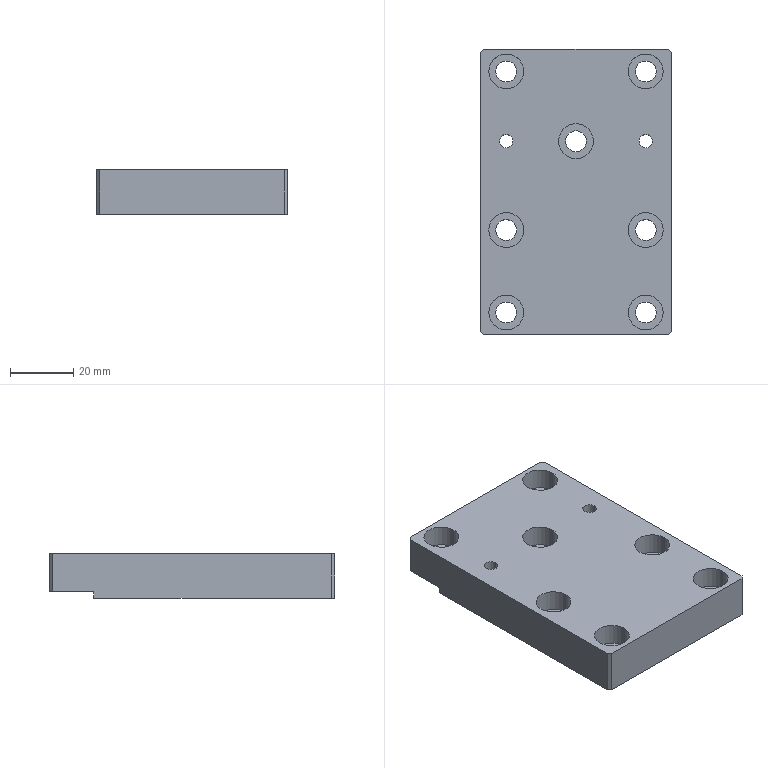Part | SolidWorks | features HoleWzd 2, Chamfer 1, Extrusion 1, ICE 1 | 1 solid | 51 faces | box 60 x 90 x 14 mm | volume 67395 mm3 | cylinder 32 | plane 19 | commonest cylinder face diameters 6.6 x14 11 x14 4.2 x4
STEP:
#1=CARTESIAN_POINT('',(-24.1,16.,-7.));
#2=VERTEX_POINT('',#1);
#3=CARTESIAN_POINT('',(-19.9,16.,-7.));
#4=VERTEX_POINT('',#3);
#5=CARTESIAN_POINT('',(-22.,16.,-7.));
#6=DIRECTION('',(0.,0.,1.));
#7=DIRECTION('',(1.,0.,0.));
#8=AXIS2_PLACEMENT_3D('',#5,#6,#7);
#9=CIRCLE('',#8,2.1);
#10=EDGE_CURVE('',#2,#4,#9,.T.);
#11=ORIENTED_EDGE('',*,*,#10,.F.);
#12=CARTESIAN_POINT('',(-24.1,16.,7.));
#13=VERTEX_POINT('',#12);
#14=CARTESIAN_POINT('',(-24.1,16.,7.));
#15=DIRECTION('',(0.,0.,1.));
#16=VECTOR('',#15,1000.);
#17=LINE('',#14,#16);
#18=EDGE_CURVE('',#2,#13,#17,.T.);
#19=ORIENTED_EDGE('',*,*,#18,.T.);
#20=CARTESIAN_POINT('',(-19.9,16.,7.));
#21=VERTEX_POINT('',#20);
#22=CARTESIAN_POINT('',(-22.,16.,7.));
#23=DIRECTION('',(0.,0.,1.));
#24=DIRECTION('',(1.,0.,0.));
#25=AXIS2_PLACEMENT_3D('',#22,#23,#24);
#26=CIRCLE('',#25,2.1);
#27=EDGE_CURVE('',#13,#21,#26,.T.);
#28=ORIENTED_EDGE('',*,*,#27,.T.);
#29=CARTESIAN_POINT('',(-19.9,16.,7.));
#30=DIRECTION('',(0.,0.,1.));
#31=VECTOR('',#30,1000.);
#32=LINE('',#29,#31);
#33=EDGE_CURVE('',#4,#21,#32,.T.);
#34=ORIENTED_EDGE('',*,*,#33,.F.);
#35=EDGE_LOOP('',(#11,#19,#28,#34));
#36=FACE_OUTER_BOUND('',#35,.T.);
#37=CARTESIAN_POINT('',(-22.,16.,7.));
#38=DIRECTION('',(0.,0.,1.));
#39=DIRECTION('',(1.,0.,0.));
#40=AXIS2_PLACEMENT_3D('',#37,#38,#39);
#41=CYLINDRICAL_SURFACE('',#40,2.1);
#42=ADVANCED_FACE('',(#36),#41,.F.);
#43=CARTESIAN_POINT('',(19.9,16.,-7.));
#44=VERTEX_POINT('',#43);
#45=CARTESIAN_POINT('',(24.1,16.,-7.));
#46=VERTEX_POINT('',#45);
#47=CARTESIAN_POINT('',(22.,16.,-7.));
#48=DIRECTION('',(0.,0.,1.));
#49=DIRECTION('',(1.,0.,0.));
#50=AXIS2_PLACEMENT_3D('',#47,#48,#49);
#51=CIRCLE('',#50,2.1);
#52=EDGE_CURVE('',#44,#46,#51,.T.);
#53=ORIENTED_EDGE('',*,*,#52,.F.);
#54=CARTESIAN_POINT('',(19.9,16.,7.));
#55=VERTEX_POINT('',#54);
#56=CARTESIAN_POINT('',(19.9,16.,7.));
#57=DIRECTION('',(0.,0.,1.));
#58=VECTOR('',#57,1000.);
#59=LINE('',#56,#58);
#60=EDGE_CURVE('',#44,#55,#59,.T.);
#61=ORIENTED_EDGE('',*,*,#60,.T.);
#62=CARTESIAN_POINT('',(24.1,16.,7.));
#63=VERTEX_POINT('',#62);
#64=CARTESIAN_POINT('',(22.,16.,7.));
#65=DIRECTION('',(0.,0.,1.));
#66=DIRECTION('',(1.,0.,0.));
#67=AXIS2_PLACEMENT_3D('',#64,#65,#66);
#68=CIRCLE('',#67,2.1);
#69=EDGE_CURVE('',#55,#63,#68,.T.);
#70=ORIENTED_EDGE('',*,*,#69,.T.);
#71=CARTESIAN_POINT('',(24.1,16.,7.));
#72=DIRECTION('',(0.,0.,1.));
#73=VECTOR('',#72,1000.);
#74=LINE('',#71,#73);
#75=EDGE_CURVE('',#46,#63,#74,.T.);
#76=ORIENTED_EDGE('',*,*,#75,.F.);
#77=EDGE_LOOP('',(#53,#61,#70,#76));
#78=FACE_OUTER_BOUND('',#77,.T.);
#79=CARTESIAN_POINT('',(22.,16.,7.));
#80=DIRECTION('',(0.,0.,1.));
#81=DIRECTION('',(1.,0.,0.));
#82=AXIS2_PLACEMENT_3D('',#79,#80,#81);
#83=CYLINDRICAL_SURFACE('',#82,2.1);
#84=ADVANCED_FACE('',(#78),#83,.F.);
#85=CARTESIAN_POINT('',(-27.5,38.,0.2));
#86=VERTEX_POINT('',#85);
#87=CARTESIAN_POINT('',(-16.5,38.,0.2));
#88=VERTEX_POINT('',#87);
#89=CARTESIAN_POINT('',(-22.,38.,0.2));
#90=DIRECTION('',(0.,0.,1.));
#91=DIRECTION('',(1.,0.,0.));
#92=AXIS2_PLACEMENT_3D('',#89,#90,#91);
#93=CIRCLE('',#92,5.5);
#94=EDGE_CURVE('',#86,#88,#93,.T.);
#95=ORIENTED_EDGE('',*,*,#94,.F.);
#96=CARTESIAN_POINT('',(-27.5,38.,7.));
#97=VERTEX_POINT('',#96);
#98=CARTESIAN_POINT('',(-27.5,38.,7.));
#99=DIRECTION('',(0.,0.,1.));
#100=VECTOR('',#99,1000.);
#101=LINE('',#98,#100);
#102=EDGE_CURVE('',#86,#97,#101,.T.);
#103=ORIENTED_EDGE('',*,*,#102,.T.);
#104=CARTESIAN_POINT('',(-16.5,38.,7.));
#105=VERTEX_POINT('',#104);
#106=CARTESIAN_POINT('',(-22.,38.,7.));
#107=DIRECTION('',(0.,0.,1.));
#108=DIRECTION('',(1.,0.,0.));
#109=AXIS2_PLACEMENT_3D('',#106,#107,#108);
#110=CIRCLE('',#109,5.5);
#111=EDGE_CURVE('',#97,#105,#110,.T.);
#112=ORIENTED_EDGE('',*,*,#111,.T.);
#113=CARTESIAN_POINT('',(-16.5,38.,7.));
#114=DIRECTION('',(0.,0.,1.));
#115=VECTOR('',#114,1000.);
#116=LINE('',#113,#115);
#117=EDGE_CURVE('',#88,#105,#116,.T.);
#118=ORIENTED_EDGE('',*,*,#117,.F.);
#119=EDGE_LOOP('',(#95,#103,#112,#118));
#120=FACE_OUTER_BOUND('',#119,.T.);
#121=CARTESIAN_POINT('',(-22.,38.,7.));
#122=DIRECTION('',(0.,0.,1.));
#123=DIRECTION('',(1.,0.,0.));
#124=AXIS2_PLACEMENT_3D('',#121,#122,#123);
#125=CYLINDRICAL_SURFACE('',#124,5.5);
#126=ADVANCED_FACE('',(#120),#125,.F.);
#127=CARTESIAN_POINT('',(-18.7,38.,-5.));
#128=VERTEX_POINT('',#127);
#129=CARTESIAN_POINT('',(-25.3,38.,-5.));
#130=VERTEX_POINT('',#129);
#131=CARTESIAN_POINT('',(-22.,38.,-5.));
#132=DIRECTION('',(0.,0.,-1.));
#133=DIRECTION('',(-1.,0.,0.));
#134=AXIS2_PLACEMENT_3D('',#131,#132,#133);
#135=CIRCLE('',#134,3.3);
#136=EDGE_CURVE('',#128,#130,#135,.T.);
#137=ORIENTED_EDGE('',*,*,#136,.T.);
#138=CARTESIAN_POINT('',(-25.3,38.,0.2));
#139=VERTEX_POINT('',#138);
#140=CARTESIAN_POINT('',(-25.3,38.,7.));
#141=DIRECTION('',(0.,0.,1.));
#142=VECTOR('',#141,1000.);
#143=LINE('',#140,#142);
#144=EDGE_CURVE('',#130,#139,#143,.T.);
#145=ORIENTED_EDGE('',*,*,#144,.T.);
#146=CARTESIAN_POINT('',(-18.7,38.,0.2));
#147=VERTEX_POINT('',#146);
#148=CARTESIAN_POINT('',(-22.,38.,0.2));
#149=DIRECTION('',(0.,0.,1.));
#150=DIRECTION('',(1.,0.,0.));
#151=AXIS2_PLACEMENT_3D('',#148,#149,#150);
#152=CIRCLE('',#151,3.3);
#153=EDGE_CURVE('',#139,#147,#152,.T.);
#154=ORIENTED_EDGE('',*,*,#153,.T.);
#155=CARTESIAN_POINT('',(-18.7,38.,7.));
#156=DIRECTION('',(0.,0.,1.));
#157=VECTOR('',#156,1000.);
#158=LINE('',#155,#157);
#159=EDGE_CURVE('',#128,#147,#158,.T.);
#160=ORIENTED_EDGE('',*,*,#159,.F.);
#161=EDGE_LOOP('',(#137,#145,#154,#160));
#162=FACE_OUTER_BOUND('',#161,.T.);
#163=CARTESIAN_POINT('',(-22.,38.,7.));
#164=DIRECTION('',(0.,0.,1.));
#165=DIRECTION('',(1.,0.,0.));
#166=AXIS2_PLACEMENT_3D('',#163,#164,#165);
#167=CYLINDRICAL_SURFACE('',#166,3.3);
#168=ADVANCED_FACE('',(#162),#167,.F.);
#169=CARTESIAN_POINT('',(16.5,38.,0.2));
#170=VERTEX_POINT('',#169);
#171=CARTESIAN_POINT('',(27.5,38.,0.2));
#172=VERTEX_POINT('',#171);
#173=CARTESIAN_POINT('',(22.,38.,0.2));
#174=DIRECTION('',(0.,0.,1.));
#175=DIRECTION('',(1.,0.,0.));
#176=AXIS2_PLACEMENT_3D('',#173,#174,#175);
#177=CIRCLE('',#176,5.5);
#178=EDGE_CURVE('',#170,#172,#177,.T.);
#179=ORIENTED_EDGE('',*,*,#178,.F.);
#180=CARTESIAN_POINT('',(16.5,38.,7.));
#181=VERTEX_POINT('',#180);
#182=CARTESIAN_POINT('',(16.5,38.,7.));
#183=DIRECTION('',(0.,0.,1.));
#184=VECTOR('',#183,1000.);
#185=LINE('',#182,#184);
#186=EDGE_CURVE('',#170,#181,#185,.T.);
#187=ORIENTED_EDGE('',*,*,#186,.T.);
#188=CARTESIAN_POINT('',(27.5,38.,7.));
#189=VERTEX_POINT('',#188);
#190=CARTESIAN_POINT('',(22.,38.,7.));
#191=DIRECTION('',(0.,0.,1.));
#192=DIRECTION('',(1.,0.,0.));
#193=AXIS2_PLACEMENT_3D('',#190,#191,#192);
#194=CIRCLE('',#193,5.5);
#195=EDGE_CURVE('',#181,#189,#194,.T.);
#196=ORIENTED_EDGE('',*,*,#195,.T.);
#197=CARTESIAN_POINT('',(27.5,38.,7.));
#198=DIRECTION('',(0.,0.,1.));
#199=VECTOR('',#198,1000.);
#200=LINE('',#197,#199);
#201=EDGE_CURVE('',#172,#189,#200,.T.);
#202=ORIENTED_EDGE('',*,*,#201,.F.);
#203=EDGE_LOOP('',(#179,#187,#196,#202));
#204=FACE_OUTER_BOUND('',#203,.T.);
#205=CARTESIAN_POINT('',(22.,38.,7.));
#206=DIRECTION('',(0.,0.,1.));
#207=DIRECTION('',(1.,0.,0.));
#208=AXIS2_PLACEMENT_3D('',#205,#206,#207);
#209=CYLINDRICAL_SURFACE('',#208,5.5);
#210=ADVANCED_FACE('',(#204),#209,.F.);
#211=CARTESIAN_POINT('',(25.3,38.,-5.));
#212=VERTEX_POINT('',#211);
#213=CARTESIAN_POINT('',(18.7,38.,-5.));
#214=VERTEX_POINT('',#213);
#215=CARTESIAN_POINT('',(22.,38.,-5.));
#216=DIRECTION('',(0.,0.,-1.));
#217=DIRECTION('',(-1.,0.,0.));
#218=AXIS2_PLACEMENT_3D('',#215,#216,#217);
#219=CIRCLE('',#218,3.3);
#220=EDGE_CURVE('',#212,#214,#219,.T.);
#221=ORIENTED_EDGE('',*,*,#220,.T.);
#222=CARTESIAN_POINT('',(18.7,38.,0.2));
#223=VERTEX_POINT('',#222);
#224=CARTESIAN_POINT('',(18.7,38.,7.));
#225=DIRECTION('',(0.,0.,1.));
#226=VECTOR('',#225,1000.);
#227=LINE('',#224,#226);
#228=EDGE_CURVE('',#214,#223,#227,.T.);
#229=ORIENTED_EDGE('',*,*,#228,.T.);
#230=CARTESIAN_POINT('',(25.3,38.,0.2));
#231=VERTEX_POINT('',#230);
#232=CARTESIAN_POINT('',(22.,38.,0.2));
#233=DIRECTION('',(0.,0.,1.));
#234=DIRECTION('',(1.,0.,0.));
#235=AXIS2_PLACEMENT_3D('',#232,#233,#234);
#236=CIRCLE('',#235,3.3);
#237=EDGE_CURVE('',#223,#231,#236,.T.);
#238=ORIENTED_EDGE('',*,*,#237,.T.);
#239=CARTESIAN_POINT('',(25.3,38.,7.));
#240=DIRECTION('',(0.,0.,1.));
#241=VECTOR('',#240,1000.);
#242=LINE('',#239,#241);
#243=EDGE_CURVE('',#212,#231,#242,.T.);
#244=ORIENTED_EDGE('',*,*,#243,.F.);
#245=EDGE_LOOP('',(#221,#229,#238,#244));
#246=FACE_OUTER_BOUND('',#245,.T.);
#247=CARTESIAN_POINT('',(22.,38.,7.));
#248=DIRECTION('',(0.,0.,1.));
#249=DIRECTION('',(1.,0.,0.));
#250=AXIS2_PLACEMENT_3D('',#247,#248,#249);
#251=CYLINDRICAL_SURFACE('',#250,3.3);
#252=ADVANCED_FACE('',(#246),#251,.F.);
#253=CARTESIAN_POINT('',(-27.5,-12.,0.2));
#254=VERTEX_POINT('',#253);
#255=CARTESIAN_POINT('',(-16.5,-12.,0.2));
#256=VERTEX_POINT('',#255);
#257=CARTESIAN_POINT('',(-22.,-12.,0.2));
#258=DIRECTION('',(0.,0.,1.));
#259=DIRECTION('',(1.,0.,0.));
#260=AXIS2_PLACEMENT_3D('',#257,#258,#259);
#261=CIRCLE('',#260,5.5);
#262=EDGE_CURVE('',#254,#256,#261,.T.);
#263=ORIENTED_EDGE('',*,*,#262,.F.);
#264=CARTESIAN_POINT('',(-27.5,-12.,7.));
#265=VERTEX_POINT('',#264);
#266=CARTESIAN_POINT('',(-27.5,-12.,7.));
#267=DIRECTION('',(0.,0.,1.));
#268=VECTOR('',#267,1000.);
#269=LINE('',#266,#268);
#270=EDGE_CURVE('',#254,#265,#269,.T.);
#271=ORIENTED_EDGE('',*,*,#270,.T.);
#272=CARTESIAN_POINT('',(-16.5,-12.,7.));
#273=VERTEX_POINT('',#272);
#274=CARTESIAN_POINT('',(-22.,-12.,7.));
#275=DIRECTION('',(0.,0.,1.));
#276=DIRECTION('',(1.,0.,0.));
#277=AXIS2_PLACEMENT_3D('',#274,#275,#276);
#278=CIRCLE('',#277,5.5);
#279=EDGE_CURVE('',#265,#273,#278,.T.);
#280=ORIENTED_EDGE('',*,*,#279,.T.);
#281=CARTESIAN_POINT('',(-16.5,-12.,7.));
#282=DIRECTION('',(0.,0.,1.));
#283=VECTOR('',#282,1000.);
#284=LINE('',#281,#283);
#285=EDGE_CURVE('',#256,#273,#284,.T.);
#286=ORIENTED_EDGE('',*,*,#285,.F.);
#287=EDGE_LOOP('',(#263,#271,#280,#286));
#288=FACE_OUTER_BOUND('',#287,.T.);
#289=CARTESIAN_POINT('',(-22.,-12.,7.));
#290=DIRECTION('',(0.,0.,1.));
#291=DIRECTION('',(1.,0.,0.));
#292=AXIS2_PLACEMENT_3D('',#289,#290,#291);
#293=CYLINDRICAL_SURFACE('',#292,5.5);
#294=ADVANCED_FACE('',(#288),#293,.F.);
#295=CARTESIAN_POINT('',(-25.3,-12.,-7.));
#296=VERTEX_POINT('',#295);
#297=CARTESIAN_POINT('',(-18.7,-12.,-7.));
#298=VERTEX_POINT('',#297);
#299=CARTESIAN_POINT('',(-22.,-12.,-7.));
#300=DIRECTION('',(0.,0.,1.));
#301=DIRECTION('',(1.,0.,0.));
#302=AXIS2_PLACEMENT_3D('',#299,#300,#301);
#303=CIRCLE('',#302,3.3);
#304=EDGE_CURVE('',#296,#298,#303,.T.);
#305=ORIENTED_EDGE('',*,*,#304,.F.);
#306=CARTESIAN_POINT('',(-25.3,-12.,0.2));
#307=VERTEX_POINT('',#306);
#308=CARTESIAN_POINT('',(-25.3,-12.,7.));
#309=DIRECTION('',(0.,0.,1.));
#310=VECTOR('',#309,1000.);
#311=LINE('',#308,#310);
#312=EDGE_CURVE('',#296,#307,#311,.T.);
#313=ORIENTED_EDGE('',*,*,#312,.T.);
#314=CARTESIAN_POINT('',(-18.7,-12.,0.2));
#315=VERTEX_POINT('',#314);
#316=CARTESIAN_POINT('',(-22.,-12.,0.2));
#317=DIRECTION('',(0.,0.,1.));
#318=DIRECTION('',(1.,0.,0.));
#319=AXIS2_PLACEMENT_3D('',#316,#317,#318);
#320=CIRCLE('',#319,3.3);
#321=EDGE_CURVE('',#307,#315,#320,.T.);
#322=ORIENTED_EDGE('',*,*,#321,.T.);
#323=CARTESIAN_POINT('',(-18.7,-12.,7.));
#324=DIRECTION('',(0.,0.,1.));
#325=VECTOR('',#324,1000.);
#326=LINE('',#323,#325);
#327=EDGE_CURVE('',#298,#315,#326,.T.);
#328=ORIENTED_EDGE('',*,*,#327,.F.);
#329=EDGE_LOOP('',(#305,#313,#322,#328));
#330=FACE_OUTER_BOUND('',#329,.T.);
#331=CARTESIAN_POINT('',(-22.,-12.,7.));
#332=DIRECTION('',(0.,0.,1.));
#333=DIRECTION('',(1.,0.,0.));
#334=AXIS2_PLACEMENT_3D('',#331,#332,#333);
#335=CYLINDRICAL_SURFACE('',#334,3.3);
#336=ADVANCED_FACE('',(#330),#335,.F.);
#337=CARTESIAN_POINT('',(16.5,-38.,0.2));
#338=VERTEX_POINT('',#337);
#339=CARTESIAN_POINT('',(27.5,-38.,0.2));
#340=VERTEX_POINT('',#339);
#341=CARTESIAN_POINT('',(22.,-38.,0.2));
#342=DIRECTION('',(0.,0.,1.));
#343=DIRECTION('',(1.,0.,0.));
#344=AXIS2_PLACEMENT_3D('',#341,#342,#343);
#345=CIRCLE('',#344,5.5);
#346=EDGE_CURVE('',#338,#340,#345,.T.);
#347=ORIENTED_EDGE('',*,*,#346,.F.);
#348=CARTESIAN_POINT('',(16.5,-38.,7.));
#349=VERTEX_POINT('',#348);
#350=CARTESIAN_POINT('',(16.5,-38.,7.));
#351=DIRECTION('',(0.,0.,1.));
#352=VECTOR('',#351,1000.);
#353=LINE('',#350,#352);
#354=EDGE_CURVE('',#338,#349,#353,.T.);
#355=ORIENTED_EDGE('',*,*,#354,.T.);
#356=CARTESIAN_POINT('',(27.5,-38.,7.));
#357=VERTEX_POINT('',#356);
#358=CARTESIAN_POINT('',(22.,-38.,7.));
#359=DIRECTION('',(0.,0.,1.));
#360=DIRECTION('',(1.,0.,0.));
#361=AXIS2_PLACEMENT_3D('',#358,#359,#360);
#362=CIRCLE('',#361,5.5);
#363=EDGE_CURVE('',#349,#357,#362,.T.);
#364=ORIENTED_EDGE('',*,*,#363,.T.);
#365=CARTESIAN_POINT('',(27.5,-38.,7.));
#366=DIRECTION('',(0.,0.,1.));
#367=VECTOR('',#366,1000.);
#368=LINE('',#365,#367);
#369=EDGE_CURVE('',#340,#357,#368,.T.);
#370=ORIENTED_EDGE('',*,*,#369,.F.);
#371=EDGE_LOOP('',(#347,#355,#364,#370));
#372=FACE_OUTER_BOUND('',#371,.T.);
#373=CARTESIAN_POINT('',(22.,-38.,7.));
#374=DIRECTION('',(0.,0.,1.));
#375=DIRECTION('',(1.,0.,0.));
#376=AXIS2_PLACEMENT_3D('',#373,#374,#375);
#377=CYLINDRICAL_SURFACE('',#376,5.5);
#378=ADVANCED_FACE('',(#372),#377,.F.);
#379=CARTESIAN_POINT('',(18.7,-38.,-7.));
#380=VERTEX_POINT('',#379);
#381=CARTESIAN_POINT('',(25.3,-38.,-7.));
#382=VERTEX_POINT('',#381);
#383=CARTESIAN_POINT('',(22.,-38.,-7.));
#384=DIRECTION('',(0.,0.,1.));
#385=DIRECTION('',(1.,0.,0.));
#386=AXIS2_PLACEMENT_3D('',#383,#384,#385);
#387=CIRCLE('',#386,3.3);
#388=EDGE_CURVE('',#380,#382,#387,.T.);
#389=ORIENTED_EDGE('',*,*,#388,.F.);
#390=CARTESIAN_POINT('',(18.7,-38.,0.2));
#391=VERTEX_POINT('',#390);
#392=CARTESIAN_POINT('',(18.7,-38.,7.));
#393=DIRECTION('',(0.,0.,1.));
#394=VECTOR('',#393,1000.);
#395=LINE('',#392,#394);
#396=EDGE_CURVE('',#380,#391,#395,.T.);
#397=ORIENTED_EDGE('',*,*,#396,.T.);
#398=CARTESIAN_POINT('',(25.3,-38.,0.2));
#399=VERTEX_POINT('',#398);
#400=CARTESIAN_POINT('',(22.,-38.,0.2));
#401=DIRECTION('',(0.,0.,1.));
#402=DIRECTION('',(1.,0.,0.));
#403=AXIS2_PLACEMENT_3D('',#400,#401,#402);
#404=CIRCLE('',#403,3.3);
#405=EDGE_CURVE('',#391,#399,#404,.T.);
#406=ORIENTED_EDGE('',*,*,#405,.T.);
#407=CARTESIAN_POINT('',(25.3,-38.,7.));
#408=DIRECTION('',(0.,0.,1.));
#409=VECTOR('',#408,1000.);
#410=LINE('',#407,#409);
#411=EDGE_CURVE('',#382,#399,#410,.T.);
#412=ORIENTED_EDGE('',*,*,#411,.F.);
#413=EDGE_LOOP('',(#389,#397,#406,#412));
#414=FACE_OUTER_BOUND('',#413,.T.);
#415=CARTESIAN_POINT('',(22.,-38.,7.));
#416=DIRECTION('',(0.,0.,1.));
#417=DIRECTION('',(1.,0.,0.));
#418=AXIS2_PLACEMENT_3D('',#415,#416,#417);
#419=CYLINDRICAL_SURFACE('',#418,3.3);
#420=ADVANCED_FACE('',(#414),#419,.F.);
#421=CARTESIAN_POINT('',(-27.5,-38.,0.2));
#422=VERTEX_POINT('',#421);
#423=CARTESIAN_POINT('',(-16.5,-38.,0.2));
#424=VERTEX_POINT('',#423);
#425=CARTESIAN_POINT('',(-22.,-38.,0.2));
#426=DIRECTION('',(0.,0.,1.));
#427=DIRECTION('',(1.,0.,0.));
#428=AXIS2_PLACEMENT_3D('',#425,#426,#427);
#429=CIRCLE('',#428,5.5);
#430=EDGE_CURVE('',#422,#424,#429,.T.);
#431=ORIENTED_EDGE('',*,*,#430,.F.);
#432=CARTESIAN_POINT('',(-27.5,-38.,7.));
#433=VERTEX_POINT('',#432);
#434=CARTESIAN_POINT('',(-27.5,-38.,7.));
#435=DIRECTION('',(0.,0.,1.));
#436=VECTOR('',#435,1000.);
#437=LINE('',#434,#436);
#438=EDGE_CURVE('',#422,#433,#437,.T.);
#439=ORIENTED_EDGE('',*,*,#438,.T.);
#440=CARTESIAN_POINT('',(-16.5,-38.,7.));
#441=VERTEX_POINT('',#440);
#442=CARTESIAN_POINT('',(-22.,-38.,7.));
#443=DIRECTION('',(0.,0.,1.));
#444=DIRECTION('',(1.,0.,0.));
#445=AXIS2_PLACEMENT_3D('',#442,#443,#444);
#446=CIRCLE('',#445,5.5);
#447=EDGE_CURVE('',#433,#441,#446,.T.);
#448=ORIENTED_EDGE('',*,*,#447,.T.);
#449=CARTESIAN_POINT('',(-16.5,-38.,7.));
#450=DIRECTION('',(0.,0.,1.));
#451=VECTOR('',#450,1000.);
#452=LINE('',#449,#451);
#453=EDGE_CURVE('',#424,#441,#452,.T.);
#454=ORIENTED_EDGE('',*,*,#453,.F.);
#455=EDGE_LOOP('',(#431,#439,#448,#454));
#456=FACE_OUTER_BOUND('',#455,.T.);
#457=CARTESIAN_POINT('',(-22.,-38.,7.));
#458=DIRECTION('',(0.,0.,1.));
#459=DIRECTION('',(1.,0.,0.));
#460=AXIS2_PLACEMENT_3D('',#457,#458,#459);
#461=CYLINDRICAL_SURFACE('',#460,5.5);
#462=ADVANCED_FACE('',(#456),#461,.F.);
#463=CARTESIAN_POINT('',(-25.3,-38.,-7.));
#464=VERTEX_POINT('',#463);
#465=CARTESIAN_POINT('',(-18.7,-38.,-7.));
#466=VERTEX_POINT('',#465);
#467=CARTESIAN_POINT('',(-22.,-38.,-7.));
#468=DIRECTION('',(0.,0.,1.));
#469=DIRECTION('',(1.,0.,0.));
#470=AXIS2_PLACEMENT_3D('',#467,#468,#469);
#471=CIRCLE('',#470,3.3);
#472=EDGE_CURVE('',#464,#466,#471,.T.);
#473=ORIENTED_EDGE('',*,*,#472,.F.);
#474=CARTESIAN_POINT('',(-25.3,-38.,0.2));
#475=VERTEX_POINT('',#474);
#476=CARTESIAN_POINT('',(-25.3,-38.,7.));
#477=DIRECTION('',(0.,0.,1.));
#478=VECTOR('',#477,1000.);
#479=LINE('',#476,#478);
#480=EDGE_CURVE('',#464,#475,#479,.T.);
#481=ORIENTED_EDGE('',*,*,#480,.T.);
#482=CARTESIAN_POINT('',(-18.7,-38.,0.2));
#483=VERTEX_POINT('',#482);
#484=CARTESIAN_POINT('',(-22.,-38.,0.2));
#485=DIRECTION('',(0.,0.,1.));
#486=DIRECTION('',(1.,0.,0.));
#487=AXIS2_PLACEMENT_3D('',#484,#485,#486);
#488=CIRCLE('',#487,3.3);
#489=EDGE_CURVE('',#475,#483,#488,.T.);
#490=ORIENTED_EDGE('',*,*,#489,.T.);
#491=CARTESIAN_POINT('',(-18.7,-38.,7.));
#492=DIRECTION('',(0.,0.,1.));
#493=VECTOR('',#492,1000.);
#494=LINE('',#491,#493);
#495=EDGE_CURVE('',#466,#483,#494,.T.);
#496=ORIENTED_EDGE('',*,*,#495,.F.);
#497=EDGE_LOOP('',(#473,#481,#490,#496));
#498=FACE_OUTER_BOUND('',#497,.T.);
#499=CARTESIAN_POINT('',(-22.,-38.,7.));
#500=DIRECTION('',(0.,0.,1.));
#501=DIRECTION('',(1.,0.,0.));
#502=AXIS2_PLACEMENT_3D('',#499,#500,#501);
#503=CYLINDRICAL_SURFACE('',#502,3.3);
#504=ADVANCED_FACE('',(#498),#503,.F.);
#505=CARTESIAN_POINT('',(16.5,-12.,0.2));
#506=VERTEX_POINT('',#505);
#507=CARTESIAN_POINT('',(27.5,-12.,0.2));
#508=VERTEX_POINT('',#507);
#509=CARTESIAN_POINT('',(22.,-12.,0.2));
#510=DIRECTION('',(0.,0.,1.));
#511=DIRECTION('',(1.,0.,0.));
#512=AXIS2_PLACEMENT_3D('',#509,#510,#511);
#513=CIRCLE('',#512,5.5);
#514=EDGE_CURVE('',#506,#508,#513,.T.);
#515=ORIENTED_EDGE('',*,*,#514,.F.);
#516=CARTESIAN_POINT('',(16.5,-12.,7.));
#517=VERTEX_POINT('',#516);
#518=CARTESIAN_POINT('',(16.5,-12.,7.));
#519=DIRECTION('',(0.,0.,1.));
#520=VECTOR('',#519,1000.);
#521=LINE('',#518,#520);
#522=EDGE_CURVE('',#506,#517,#521,.T.);
#523=ORIENTED_EDGE('',*,*,#522,.T.);
#524=CARTESIAN_POINT('',(27.5,-12.,7.));
#525=VERTEX_POINT('',#524);
#526=CARTESIAN_POINT('',(22.,-12.,7.));
#527=DIRECTION('',(0.,0.,1.));
#528=DIRECTION('',(1.,0.,0.));
#529=AXIS2_PLACEMENT_3D('',#526,#527,#528);
#530=CIRCLE('',#529,5.5);
#531=EDGE_CURVE('',#517,#525,#530,.T.);
#532=ORIENTED_EDGE('',*,*,#531,.T.);
#533=CARTESIAN_POINT('',(27.5,-12.,7.));
#534=DIRECTION('',(0.,0.,1.));
#535=VECTOR('',#534,1000.);
#536=LINE('',#533,#535);
#537=EDGE_CURVE('',#508,#525,#536,.T.);
#538=ORIENTED_EDGE('',*,*,#537,.F.);
#539=EDGE_LOOP('',(#515,#523,#532,#538));
#540=FACE_OUTER_BOUND('',#539,.T.);
#541=CARTESIAN_POINT('',(22.,-12.,7.));
#542=DIRECTION('',(0.,0.,1.));
#543=DIRECTION('',(1.,0.,0.));
#544=AXIS2_PLACEMENT_3D('',#541,#542,#543);
#545=CYLINDRICAL_SURFACE('',#544,5.5);
#546=ADVANCED_FACE('',(#540),#545,.F.);
#547=CARTESIAN_POINT('',(18.7,-12.,-7.));
#548=VERTEX_POINT('',#547);
#549=CARTESIAN_POINT('',(25.3,-12.,-7.));
#550=VERTEX_POINT('',#549);
#551=CARTESIAN_POINT('',(22.,-12.,-7.));
#552=DIRECTION('',(0.,0.,1.));
#553=DIRECTION('',(1.,0.,0.));
#554=AXIS2_PLACEMENT_3D('',#551,#552,#553);
#555=CIRCLE('',#554,3.3);
#556=EDGE_CURVE('',#548,#550,#555,.T.);
#557=ORIENTED_EDGE('',*,*,#556,.F.);
#558=CARTESIAN_POINT('',(18.7,-12.,0.2));
#559=VERTEX_POINT('',#558);
#560=CARTESIAN_POINT('',(18.7,-12.,7.));
#561=DIRECTION('',(0.,0.,1.));
#562=VECTOR('',#561,1000.);
#563=LINE('',#560,#562);
#564=EDGE_CURVE('',#548,#559,#563,.T.);
#565=ORIENTED_EDGE('',*,*,#564,.T.);
#566=CARTESIAN_POINT('',(25.3,-12.,0.2));
#567=VERTEX_POINT('',#566);
#568=CARTESIAN_POINT('',(22.,-12.,0.2));
#569=DIRECTION('',(0.,0.,1.));
#570=DIRECTION('',(1.,0.,0.));
#571=AXIS2_PLACEMENT_3D('',#568,#569,#570);
#572=CIRCLE('',#571,3.3);
#573=EDGE_CURVE('',#559,#567,#572,.T.);
#574=ORIENTED_EDGE('',*,*,#573,.T.);
#575=CARTESIAN_POINT('',(25.3,-12.,7.));
#576=DIRECTION('',(0.,0.,1.));
#577=VECTOR('',#576,1000.);
#578=LINE('',#575,#577);
#579=EDGE_CURVE('',#550,#567,#578,.T.);
#580=ORIENTED_EDGE('',*,*,#579,.F.);
#581=EDGE_LOOP('',(#557,#565,#574,#580));
#582=FACE_OUTER_BOUND('',#581,.T.);
#583=CARTESIAN_POINT('',(22.,-12.,7.));
#584=DIRECTION('',(0.,0.,1.));
#585=DIRECTION('',(1.,0.,0.));
#586=AXIS2_PLACEMENT_3D('',#583,#584,#585);
#587=CYLINDRICAL_SURFACE('',#586,3.3);
#588=ADVANCED_FACE('',(#582),#587,.F.);
#589=CARTESIAN_POINT('',(-5.5,16.,0.2));
#590=VERTEX_POINT('',#589);
#591=CARTESIAN_POINT('',(5.5,16.,0.2));
#592=VERTEX_POINT('',#591);
#593=CARTESIAN_POINT('',(0.,16.,0.2));
#594=DIRECTION('',(0.,0.,1.));
#595=DIRECTION('',(1.,0.,0.));
#596=AXIS2_PLACEMENT_3D('',#593,#594,#595);
#597=CIRCLE('',#596,5.5);
#598=EDGE_CURVE('',#590,#592,#597,.T.);
#599=ORIENTED_EDGE('',*,*,#598,.F.);
#600=CARTESIAN_POINT('',(-5.5,16.,7.));
#601=VERTEX_POINT('',#600);
#602=CARTESIAN_POINT('',(-5.5,16.,7.));
#603=DIRECTION('',(0.,0.,1.));
#604=VECTOR('',#603,1000.);
#605=LINE('',#602,#604);
#606=EDGE_CURVE('',#590,#601,#605,.T.);
#607=ORIENTED_EDGE('',*,*,#606,.T.);
#608=CARTESIAN_POINT('',(5.5,16.,7.));
#609=VERTEX_POINT('',#608);
#610=CARTESIAN_POINT('',(0.,16.,7.));
#611=DIRECTION('',(0.,0.,1.));
#612=DIRECTION('',(1.,0.,0.));
#613=AXIS2_PLACEMENT_3D('',#610,#611,#612);
#614=CIRCLE('',#613,5.5);
#615=EDGE_CURVE('',#601,#609,#614,.T.);
#616=ORIENTED_EDGE('',*,*,#615,.T.);
#617=CARTESIAN_POINT('',(5.5,16.,7.));
#618=DIRECTION('',(0.,0.,1.));
#619=VECTOR('',#618,1000.);
#620=LINE('',#617,#619);
#621=EDGE_CURVE('',#592,#609,#620,.T.);
#622=ORIENTED_EDGE('',*,*,#621,.F.);
#623=EDGE_LOOP('',(#599,#607,#616,#622));
#624=FACE_OUTER_BOUND('',#623,.T.);
#625=CARTESIAN_POINT('',(0.,16.,7.));
#626=DIRECTION('',(0.,0.,1.));
#627=DIRECTION('',(1.,0.,0.));
#628=AXIS2_PLACEMENT_3D('',#625,#626,#627);
#629=CYLINDRICAL_SURFACE('',#628,5.5);
#630=ADVANCED_FACE('',(#624),#629,.F.);
#631=CARTESIAN_POINT('',(-3.3,16.,-7.));
#632=VERTEX_POINT('',#631);
#633=CARTESIAN_POINT('',(3.3,16.,-7.));
#634=VERTEX_POINT('',#633);
#635=CARTESIAN_POINT('',(0.,16.,-7.));
#636=DIRECTION('',(0.,0.,1.));
#637=DIRECTION('',(1.,0.,0.));
#638=AXIS2_PLACEMENT_3D('',#635,#636,#637);
#639=CIRCLE('',#638,3.3);
#640=EDGE_CURVE('',#632,#634,#639,.T.);
#641=ORIENTED_EDGE('',*,*,#640,.F.);
#642=CARTESIAN_POINT('',(-3.3,16.,0.2));
#643=VERTEX_POINT('',#642);
#644=CARTESIAN_POINT('',(-3.3,16.,7.));
#645=DIRECTION('',(0.,0.,1.));
#646=VECTOR('',#645,1000.);
#647=LINE('',#644,#646);
#648=EDGE_CURVE('',#632,#643,#647,.T.);
#649=ORIENTED_EDGE('',*,*,#648,.T.);
#650=CARTESIAN_POINT('',(3.3,16.,0.2));
#651=VERTEX_POINT('',#650);
#652=CARTESIAN_POINT('',(0.,16.,0.2));
#653=DIRECTION('',(0.,0.,1.));
#654=DIRECTION('',(1.,0.,0.));
#655=AXIS2_PLACEMENT_3D('',#652,#653,#654);
#656=CIRCLE('',#655,3.3);
#657=EDGE_CURVE('',#643,#651,#656,.T.);
#658=ORIENTED_EDGE('',*,*,#657,.T.);
#659=CARTESIAN_POINT('',(3.3,16.,7.));
#660=DIRECTION('',(0.,0.,1.));
#661=VECTOR('',#660,1000.);
#662=LINE('',#659,#661);
#663=EDGE_CURVE('',#634,#651,#662,.T.);
#664=ORIENTED_EDGE('',*,*,#663,.F.);
#665=EDGE_LOOP('',(#641,#649,#658,#664));
#666=FACE_OUTER_BOUND('',#665,.T.);
#667=CARTESIAN_POINT('',(0.,16.,7.));
#668=DIRECTION('',(0.,0.,1.));
#669=DIRECTION('',(1.,0.,0.));
#670=AXIS2_PLACEMENT_3D('',#667,#668,#669);
#671=CYLINDRICAL_SURFACE('',#670,3.3);
#672=ADVANCED_FACE('',(#666),#671,.F.);
#673=CARTESIAN_POINT('',(29.,45.,7.));
#674=VERTEX_POINT('',#673);
#675=CARTESIAN_POINT('',(-29.,45.,7.));
#676=VERTEX_POINT('',#675);
#677=CARTESIAN_POINT('',(-30.,45.,7.));
#678=DIRECTION('',(-1.,0.,0.));
#679=VECTOR('',#678,1000.);
#680=LINE('',#677,#679);
#681=EDGE_CURVE('',#674,#676,#680,.T.);
#682=ORIENTED_EDGE('',*,*,#681,.F.);
#683=CARTESIAN_POINT('',(29.,45.,-5.));
#684=VERTEX_POINT('',#683);
#685=CARTESIAN_POINT('',(29.,45.,7.));
#686=DIRECTION('',(0.,0.,-1.));
#687=VECTOR('',#686,1000.);
#688=LINE('',#685,#687);
#689=EDGE_CURVE('',#674,#684,#688,.T.);
#690=ORIENTED_EDGE('',*,*,#689,.T.);
#691=CARTESIAN_POINT('',(-29.,45.,-5.));
#692=VERTEX_POINT('',#691);
#693=CARTESIAN_POINT('',(30.,45.,-5.));
#694=DIRECTION('',(1.,0.,0.));
#695=VECTOR('',#694,1000.);
#696=LINE('',#693,#695);
#697=EDGE_CURVE('',#692,#684,#696,.T.);
#698=ORIENTED_EDGE('',*,*,#697,.F.);
#699=CARTESIAN_POINT('',(-29.,45.,7.));
#700=DIRECTION('',(0.,0.,1.));
#701=VECTOR('',#700,1000.);
#702=LINE('',#699,#701);
#703=EDGE_CURVE('',#692,#676,#702,.T.);
#704=ORIENTED_EDGE('',*,*,#703,.T.);
#705=EDGE_LOOP('',(#682,#690,#698,#704));
#706=FACE_OUTER_BOUND('',#705,.T.);
#707=CARTESIAN_POINT('',(-30.,45.,7.));
#708=DIRECTION('',(0.,-1.,0.));
#709=DIRECTION('',(0.,0.,-1.));
#710=AXIS2_PLACEMENT_3D('',#707,#708,#709);
#711=PLANE('',#710);
#712=ADVANCED_FACE('',(#706),#711,.F.);
#713=CARTESIAN_POINT('',(30.,-44.,7.));
#714=VERTEX_POINT('',#713);
#715=CARTESIAN_POINT('',(30.,44.,7.));
#716=VERTEX_POINT('',#715);
#717=CARTESIAN_POINT('',(30.,-45.,7.));
#718=DIRECTION('',(0.,1.,0.));
#719=VECTOR('',#718,1000.);
#720=LINE('',#717,#719);
#721=EDGE_CURVE('',#714,#716,#720,.T.);
#722=ORIENTED_EDGE('',*,*,#721,.F.);
#723=CARTESIAN_POINT('',(30.,-44.,-7.));
#724=VERTEX_POINT('',#723);
#725=CARTESIAN_POINT('',(30.,-44.,7.));
#726=DIRECTION('',(0.,0.,-1.));
#727=VECTOR('',#726,1000.);
#728=LINE('',#725,#727);
#729=EDGE_CURVE('',#714,#724,#728,.T.);
#730=ORIENTED_EDGE('',*,*,#729,.T.);
#731=CARTESIAN_POINT('',(30.,31.,-7.));
#732=VERTEX_POINT('',#731);
#733=CARTESIAN_POINT('',(30.,-45.,-7.));
#734=DIRECTION('',(0.,1.,0.));
#735=VECTOR('',#734,1000.);
#736=LINE('',#733,#735);
#737=EDGE_CURVE('',#724,#732,#736,.T.);
#738=ORIENTED_EDGE('',*,*,#737,.T.);
#739=CARTESIAN_POINT('',(30.,31.,-5.));
#740=VERTEX_POINT('',#739);
#741=CARTESIAN_POINT('',(30.,31.,-5.));
#742=DIRECTION('',(0.,0.,-1.));
#743=VECTOR('',#742,1000.);
#744=LINE('',#741,#743);
#745=EDGE_CURVE('',#740,#732,#744,.T.);
#746=ORIENTED_EDGE('',*,*,#745,.F.);
#747=CARTESIAN_POINT('',(30.,44.,-5.));
#748=VERTEX_POINT('',#747);
#749=CARTESIAN_POINT('',(30.,45.,-5.));
#750=DIRECTION('',(0.,-1.,0.));
#751=VECTOR('',#750,1000.);
#752=LINE('',#749,#751);
#753=EDGE_CURVE('',#748,#740,#752,.T.);
#754=ORIENTED_EDGE('',*,*,#753,.F.);
#755=CARTESIAN_POINT('',(30.,44.,7.));
#756=DIRECTION('',(0.,0.,1.));
#757=VECTOR('',#756,1000.);
#758=LINE('',#755,#757);
#759=EDGE_CURVE('',#748,#716,#758,.T.);
#760=ORIENTED_EDGE('',*,*,#759,.T.);
#761=EDGE_LOOP('',(#722,#730,#738,#746,#754,#760));
#762=FACE_OUTER_BOUND('',#761,.T.);
#763=CARTESIAN_POINT('',(30.,-45.,7.));
#764=DIRECTION('',(-1.,0.,0.));
#765=DIRECTION('',(0.,0.,1.));
#766=AXIS2_PLACEMENT_3D('',#763,#764,#765);
#767=PLANE('',#766);
#768=ADVANCED_FACE('',(#762),#767,.F.);
#769=CARTESIAN_POINT('',(-30.,31.,-7.));
#770=VERTEX_POINT('',#769);
#771=CARTESIAN_POINT('',(-30.,-44.,-7.));
#772=VERTEX_POINT('',#771);
#773=CARTESIAN_POINT('',(-30.,-45.,-7.));
#774=DIRECTION('',(0.,-1.,0.));
#775=VECTOR('',#774,1000.);
#776=LINE('',#773,#775);
#777=EDGE_CURVE('',#770,#772,#776,.T.);
#778=ORIENTED_EDGE('',*,*,#777,.T.);
#779=CARTESIAN_POINT('',(-30.,-44.,7.));
#780=VERTEX_POINT('',#779);
#781=CARTESIAN_POINT('',(-30.,-44.,7.));
#782=DIRECTION('',(0.,0.,1.));
#783=VECTOR('',#782,1000.);
#784=LINE('',#781,#783);
#785=EDGE_CURVE('',#772,#780,#784,.T.);
#786=ORIENTED_EDGE('',*,*,#785,.T.);
#787=CARTESIAN_POINT('',(-30.,44.,7.));
#788=VERTEX_POINT('',#787);
#789=CARTESIAN_POINT('',(-30.,-45.,7.));
#790=DIRECTION('',(0.,-1.,0.));
#791=VECTOR('',#790,1000.);
#792=LINE('',#789,#791);
#793=EDGE_CURVE('',#788,#780,#792,.T.);
#794=ORIENTED_EDGE('',*,*,#793,.F.);
#795=CARTESIAN_POINT('',(-30.,44.,-5.));
#796=VERTEX_POINT('',#795);
#797=CARTESIAN_POINT('',(-30.,44.,7.));
#798=DIRECTION('',(0.,0.,-1.));
#799=VECTOR('',#798,1000.);
#800=LINE('',#797,#799);
#801=EDGE_CURVE('',#788,#796,#800,.T.);
#802=ORIENTED_EDGE('',*,*,#801,.T.);
#803=CARTESIAN_POINT('',(-30.,31.,-5.));
#804=VERTEX_POINT('',#803);
#805=CARTESIAN_POINT('',(-30.,45.,-5.));
#806=DIRECTION('',(0.,1.,0.));
#807=VECTOR('',#806,1000.);
#808=LINE('',#805,#807);
#809=EDGE_CURVE('',#804,#796,#808,.T.);
#810=ORIENTED_EDGE('',*,*,#809,.F.);
#811=CARTESIAN_POINT('',(-30.,31.,-5.));
#812=DIRECTION('',(0.,0.,-1.));
#813=VECTOR('',#812,1000.);
#814=LINE('',#811,#813);
#815=EDGE_CURVE('',#804,#770,#814,.T.);
#816=ORIENTED_EDGE('',*,*,#815,.T.);
#817=EDGE_LOOP('',(#778,#786,#794,#802,#810,#816));
#818=FACE_OUTER_BOUND('',#817,.T.);
#819=CARTESIAN_POINT('',(-30.,-45.,7.));
#820=DIRECTION('',(1.,0.,0.));
#821=DIRECTION('',(0.,0.,-1.));
#822=AXIS2_PLACEMENT_3D('',#819,#820,#821);
#823=PLANE('',#822);
#824=ADVANCED_FACE('',(#818),#823,.F.);
#825=CARTESIAN_POINT('',(-29.,-45.,-7.));
#826=VERTEX_POINT('',#825);
#827=CARTESIAN_POINT('',(29.,-45.,-7.));
#828=VERTEX_POINT('',#827);
#829=CARTESIAN_POINT('',(-30.,-45.,-7.));
#830=DIRECTION('',(1.,0.,0.));
#831=VECTOR('',#830,1000.);
#832=LINE('',#829,#831);
#833=EDGE_CURVE('',#826,#828,#832,.T.);
#834=ORIENTED_EDGE('',*,*,#833,.T.);
#835=CARTESIAN_POINT('',(29.,-45.,7.));
#836=VERTEX_POINT('',#835);
#837=CARTESIAN_POINT('',(29.,-45.,7.));
#838=DIRECTION('',(0.,0.,1.));
#839=VECTOR('',#838,1000.);
#840=LINE('',#837,#839);
#841=EDGE_CURVE('',#828,#836,#840,.T.);
#842=ORIENTED_EDGE('',*,*,#841,.T.);
#843=CARTESIAN_POINT('',(-29.,-45.,7.));
#844=VERTEX_POINT('',#843);
#845=CARTESIAN_POINT('',(-30.,-45.,7.));
#846=DIRECTION('',(1.,0.,0.));
#847=VECTOR('',#846,1000.);
#848=LINE('',#845,#847);
#849=EDGE_CURVE('',#844,#836,#848,.T.);
#850=ORIENTED_EDGE('',*,*,#849,.F.);
#851=CARTESIAN_POINT('',(-29.,-45.,7.));
#852=DIRECTION('',(0.,0.,-1.));
#853=VECTOR('',#852,1000.);
#854=LINE('',#851,#853);
#855=EDGE_CURVE('',#844,#826,#854,.T.);
#856=ORIENTED_EDGE('',*,*,#855,.T.);
#857=EDGE_LOOP('',(#834,#842,#850,#856));
#858=FACE_OUTER_BOUND('',#857,.T.);
#859=CARTESIAN_POINT('',(-30.,-45.,7.));
#860=DIRECTION('',(0.,1.,0.));
#861=DIRECTION('',(0.,0.,1.));
#862=AXIS2_PLACEMENT_3D('',#859,#860,#861);
#863=PLANE('',#862);
#864=ADVANCED_FACE('',(#858),#863,.F.);
#865=CARTESIAN_POINT('',(-22.,16.,7.));
#866=DIRECTION('',(0.,0.,1.));
#867=DIRECTION('',(1.,0.,0.));
#868=AXIS2_PLACEMENT_3D('',#865,#866,#867);
#869=CIRCLE('',#868,2.1);
#870=EDGE_CURVE('',#21,#13,#869,.T.);
#871=ORIENTED_EDGE('',*,*,#870,.F.);
#872=ORIENTED_EDGE('',*,*,#27,.F.);
#873=EDGE_LOOP('',(#871,#872));
#874=FACE_BOUND('',#873,.T.);
#875=CARTESIAN_POINT('',(22.,16.,7.));
#876=DIRECTION('',(0.,0.,1.));
#877=DIRECTION('',(1.,0.,0.));
#878=AXIS2_PLACEMENT_3D('',#875,#876,#877);
#879=CIRCLE('',#878,2.1);
#880=EDGE_CURVE('',#63,#55,#879,.T.);
#881=ORIENTED_EDGE('',*,*,#880,.F.);
#882=ORIENTED_EDGE('',*,*,#69,.F.);
#883=EDGE_LOOP('',(#881,#882));
#884=FACE_BOUND('',#883,.T.);
#885=CARTESIAN_POINT('',(-22.,38.,7.));
#886=DIRECTION('',(0.,0.,1.));
#887=DIRECTION('',(1.,0.,0.));
#888=AXIS2_PLACEMENT_3D('',#885,#886,#887);
#889=CIRCLE('',#888,5.5);
#890=EDGE_CURVE('',#105,#97,#889,.T.);
#891=ORIENTED_EDGE('',*,*,#890,.F.);
#892=ORIENTED_EDGE('',*,*,#111,.F.);
#893=EDGE_LOOP('',(#891,#892));
#894=FACE_BOUND('',#893,.T.);
#895=CARTESIAN_POINT('',(22.,38.,7.));
#896=DIRECTION('',(0.,0.,1.));
#897=DIRECTION('',(1.,0.,0.));
#898=AXIS2_PLACEMENT_3D('',#895,#896,#897);
#899=CIRCLE('',#898,5.5);
#900=EDGE_CURVE('',#189,#181,#899,.T.);
#901=ORIENTED_EDGE('',*,*,#900,.F.);
#902=ORIENTED_EDGE('',*,*,#195,.F.);
#903=EDGE_LOOP('',(#901,#902));
#904=FACE_BOUND('',#903,.T.);
#905=CARTESIAN_POINT('',(-22.,-12.,7.));
#906=DIRECTION('',(0.,0.,1.));
#907=DIRECTION('',(1.,0.,0.));
#908=AXIS2_PLACEMENT_3D('',#905,#906,#907);
#909=CIRCLE('',#908,5.5);
#910=EDGE_CURVE('',#273,#265,#909,.T.);
#911=ORIENTED_EDGE('',*,*,#910,.F.);
#912=ORIENTED_EDGE('',*,*,#279,.F.);
#913=EDGE_LOOP('',(#911,#912));
#914=FACE_BOUND('',#913,.T.);
#915=CARTESIAN_POINT('',(22.,-38.,7.));
#916=DIRECTION('',(0.,0.,1.));
#917=DIRECTION('',(1.,0.,0.));
#918=AXIS2_PLACEMENT_3D('',#915,#916,#917);
#919=CIRCLE('',#918,5.5);
#920=EDGE_CURVE('',#357,#349,#919,.T.);
#921=ORIENTED_EDGE('',*,*,#920,.F.);
#922=ORIENTED_EDGE('',*,*,#363,.F.);
#923=EDGE_LOOP('',(#921,#922));
#924=FACE_BOUND('',#923,.T.);
#925=CARTESIAN_POINT('',(-22.,-38.,7.));
#926=DIRECTION('',(0.,0.,1.));
#927=DIRECTION('',(1.,0.,0.));
#928=AXIS2_PLACEMENT_3D('',#925,#926,#927);
#929=CIRCLE('',#928,5.5);
#930=EDGE_CURVE('',#441,#433,#929,.T.);
#931=ORIENTED_EDGE('',*,*,#930,.F.);
#932=ORIENTED_EDGE('',*,*,#447,.F.);
#933=EDGE_LOOP('',(#931,#932));
#934=FACE_BOUND('',#933,.T.);
#935=CARTESIAN_POINT('',(22.,-12.,7.));
#936=DIRECTION('',(0.,0.,1.));
#937=DIRECTION('',(1.,0.,0.));
#938=AXIS2_PLACEMENT_3D('',#935,#936,#937);
#939=CIRCLE('',#938,5.5);
#940=EDGE_CURVE('',#525,#517,#939,.T.);
#941=ORIENTED_EDGE('',*,*,#940,.F.);
#942=ORIENTED_EDGE('',*,*,#531,.F.);
#943=EDGE_LOOP('',(#941,#942));
#944=FACE_BOUND('',#943,.T.);
#945=CARTESIAN_POINT('',(0.,16.,7.));
#946=DIRECTION('',(0.,0.,1.));
#947=DIRECTION('',(1.,0.,0.));
#948=AXIS2_PLACEMENT_3D('',#945,#946,#947);
#949=CIRCLE('',#948,5.5);
#950=EDGE_CURVE('',#609,#601,#949,.T.);
#951=ORIENTED_EDGE('',*,*,#950,.F.);
#952=ORIENTED_EDGE('',*,*,#615,.F.);
#953=EDGE_LOOP('',(#951,#952));
#954=FACE_BOUND('',#953,.T.);
#955=ORIENTED_EDGE('',*,*,#849,.T.);
#956=CARTESIAN_POINT('',(30.,-44.,7.));
#957=DIRECTION('',(0.7071,0.7071,0.));
#958=VECTOR('',#957,1000.);
#959=LINE('',#956,#958);
#960=EDGE_CURVE('',#836,#714,#959,.T.);
#961=ORIENTED_EDGE('',*,*,#960,.T.);
#962=ORIENTED_EDGE('',*,*,#721,.T.);
#963=CARTESIAN_POINT('',(29.,45.,7.));
#964=DIRECTION('',(-0.7071,0.7071,0.));
#965=VECTOR('',#964,1000.);
#966=LINE('',#963,#965);
#967=EDGE_CURVE('',#716,#674,#966,.T.);
#968=ORIENTED_EDGE('',*,*,#967,.T.);
#969=ORIENTED_EDGE('',*,*,#681,.T.);
#970=CARTESIAN_POINT('',(-30.,44.,7.));
#971=DIRECTION('',(-0.7071,-0.7071,0.));
#972=VECTOR('',#971,1000.);
#973=LINE('',#970,#972);
#974=EDGE_CURVE('',#676,#788,#973,.T.);
#975=ORIENTED_EDGE('',*,*,#974,.T.);
#976=ORIENTED_EDGE('',*,*,#793,.T.);
#977=CARTESIAN_POINT('',(-29.,-45.,7.));
#978=DIRECTION('',(0.7071,-0.7071,0.));
#979=VECTOR('',#978,1000.);
#980=LINE('',#977,#979);
#981=EDGE_CURVE('',#780,#844,#980,.T.);
#982=ORIENTED_EDGE('',*,*,#981,.T.);
#983=EDGE_LOOP('',(#955,#961,#962,#968,#969,#975,#976,#982));
#984=FACE_OUTER_BOUND('',#983,.T.);
#985=CARTESIAN_POINT('',(0.,0.,7.));
#986=DIRECTION('',(0.,0.,-1.));
#987=DIRECTION('',(-1.,0.,0.));
#988=AXIS2_PLACEMENT_3D('',#985,#986,#987);
#989=PLANE('',#988);
#990=ADVANCED_FACE('',(#874,#884,#894,#904,#914,#924,#934,#944,#954,#984),#989,.F.);
#991=CARTESIAN_POINT('',(-22.,16.,-7.));
#992=DIRECTION('',(0.,0.,1.));
#993=DIRECTION('',(1.,0.,0.));
#994=AXIS2_PLACEMENT_3D('',#991,#992,#993);
#995=CIRCLE('',#994,2.1);
#996=EDGE_CURVE('',#4,#2,#995,.T.);
#997=ORIENTED_EDGE('',*,*,#996,.T.);
#998=ORIENTED_EDGE('',*,*,#10,.T.);
#999=EDGE_LOOP('',(#997,#998));
#1000=FACE_BOUND('',#999,.T.);
#1001=CARTESIAN_POINT('',(22.,16.,-7.));
#1002=DIRECTION('',(0.,0.,1.));
#1003=DIRECTION('',(1.,0.,0.));
#1004=AXIS2_PLACEMENT_3D('',#1001,#1002,#1003);
#1005=CIRCLE('',#1004,2.1);
#1006=EDGE_CURVE('',#46,#44,#1005,.T.);
#1007=ORIENTED_EDGE('',*,*,#1006,.T.);
#1008=ORIENTED_EDGE('',*,*,#52,.T.);
#1009=EDGE_LOOP('',(#1007,#1008));
#1010=FACE_BOUND('',#1009,.T.);
#1011=CARTESIAN_POINT('',(-22.,-12.,-7.));
#1012=DIRECTION('',(0.,0.,1.));
#1013=DIRECTION('',(1.,0.,0.));
#1014=AXIS2_PLACEMENT_3D('',#1011,#1012,#1013);
#1015=CIRCLE('',#1014,3.3);
#1016=EDGE_CURVE('',#298,#296,#1015,.T.);
#1017=ORIENTED_EDGE('',*,*,#1016,.T.);
#1018=ORIENTED_EDGE('',*,*,#304,.T.);
#1019=EDGE_LOOP('',(#1017,#1018));
#1020=FACE_BOUND('',#1019,.T.);
#1021=CARTESIAN_POINT('',(22.,-38.,-7.));
#1022=DIRECTION('',(0.,0.,1.));
#1023=DIRECTION('',(1.,0.,0.));
#1024=AXIS2_PLACEMENT_3D('',#1021,#1022,#1023);
#1025=CIRCLE('',#1024,3.3);
#1026=EDGE_CURVE('',#382,#380,#1025,.T.);
#1027=ORIENTED_EDGE('',*,*,#1026,.T.);
#1028=ORIENTED_EDGE('',*,*,#388,.T.);
#1029=EDGE_LOOP('',(#1027,#1028));
#1030=FACE_BOUND('',#1029,.T.);
#1031=CARTESIAN_POINT('',(-22.,-38.,-7.));
#1032=DIRECTION('',(0.,0.,1.));
#1033=DIRECTION('',(1.,0.,0.));
#1034=AXIS2_PLACEMENT_3D('',#1031,#1032,#1033);
#1035=CIRCLE('',#1034,3.3);
#1036=EDGE_CURVE('',#466,#464,#1035,.T.);
#1037=ORIENTED_EDGE('',*,*,#1036,.T.);
#1038=ORIENTED_EDGE('',*,*,#472,.T.);
#1039=EDGE_LOOP('',(#1037,#1038));
#1040=FACE_BOUND('',#1039,.T.);
#1041=CARTESIAN_POINT('',(22.,-12.,-7.));
#1042=DIRECTION('',(0.,0.,1.));
#1043=DIRECTION('',(1.,0.,0.));
#1044=AXIS2_PLACEMENT_3D('',#1041,#1042,#1043);
#1045=CIRCLE('',#1044,3.3);
#1046=EDGE_CURVE('',#550,#548,#1045,.T.);
#1047=ORIENTED_EDGE('',*,*,#1046,.T.);
#1048=ORIENTED_EDGE('',*,*,#556,.T.);
#1049=EDGE_LOOP('',(#1047,#1048));
#1050=FACE_BOUND('',#1049,.T.);
#1051=CARTESIAN_POINT('',(0.,16.,-7.));
#1052=DIRECTION('',(0.,0.,1.));
#1053=DIRECTION('',(1.,0.,0.));
#1054=AXIS2_PLACEMENT_3D('',#1051,#1052,#1053);
#1055=CIRCLE('',#1054,3.3);
#1056=EDGE_CURVE('',#634,#632,#1055,.T.);
#1057=ORIENTED_EDGE('',*,*,#1056,.T.);
#1058=ORIENTED_EDGE('',*,*,#640,.T.);
#1059=EDGE_LOOP('',(#1057,#1058));
#1060=FACE_BOUND('',#1059,.T.);
#1061=ORIENTED_EDGE('',*,*,#737,.F.);
#1062=CARTESIAN_POINT('',(37.,-37.,-7.));
#1063=DIRECTION('',(-0.7071,-0.7071,0.));
#1064=VECTOR('',#1063,1000.);
#1065=LINE('',#1062,#1064);
#1066=EDGE_CURVE('',#724,#828,#1065,.T.);
#1067=ORIENTED_EDGE('',*,*,#1066,.T.);
#1068=ORIENTED_EDGE('',*,*,#833,.F.);
#1069=CARTESIAN_POINT('',(-37.,-37.,-7.));
#1070=DIRECTION('',(-0.7071,0.7071,0.));
#1071=VECTOR('',#1070,1000.);
#1072=LINE('',#1069,#1071);
#1073=EDGE_CURVE('',#826,#772,#1072,.T.);
#1074=ORIENTED_EDGE('',*,*,#1073,.T.);
#1075=ORIENTED_EDGE('',*,*,#777,.F.);
#1076=CARTESIAN_POINT('',(30.,31.,-7.));
#1077=DIRECTION('',(-1.,0.,0.));
#1078=VECTOR('',#1077,1000.);
#1079=LINE('',#1076,#1078);
#1080=EDGE_CURVE('',#732,#770,#1079,.T.);
#1081=ORIENTED_EDGE('',*,*,#1080,.F.);
#1082=EDGE_LOOP('',(#1061,#1067,#1068,#1074,#1075,#1081));
#1083=FACE_OUTER_BOUND('',#1082,.T.);
#1084=CARTESIAN_POINT('',(0.,0.,-7.));
#1085=DIRECTION('',(0.,0.,-1.));
#1086=DIRECTION('',(-1.,0.,0.));
#1087=AXIS2_PLACEMENT_3D('',#1084,#1085,#1086);
#1088=PLANE('',#1087);
#1089=ADVANCED_FACE('',(#1000,#1010,#1020,#1030,#1040,#1050,#1060,#1083),#1088,.T.);
#1090=ORIENTED_EDGE('',*,*,#1080,.T.);
#1091=ORIENTED_EDGE('',*,*,#815,.F.);
#1092=CARTESIAN_POINT('',(30.,31.,-5.));
#1093=DIRECTION('',(-1.,0.,0.));
#1094=VECTOR('',#1093,1000.);
#1095=LINE('',#1092,#1094);
#1096=EDGE_CURVE('',#740,#804,#1095,.T.);
#1097=ORIENTED_EDGE('',*,*,#1096,.F.);
#1098=ORIENTED_EDGE('',*,*,#745,.T.);
#1099=EDGE_LOOP('',(#1090,#1091,#1097,#1098));
#1100=FACE_OUTER_BOUND('',#1099,.T.);
#1101=CARTESIAN_POINT('',(30.,31.,-5.));
#1102=DIRECTION('',(0.,-1.,0.));
#1103=DIRECTION('',(0.,0.,-1.));
#1104=AXIS2_PLACEMENT_3D('',#1101,#1102,#1103);
#1105=PLANE('',#1104);
#1106=ADVANCED_FACE('',(#1100),#1105,.F.);
#1107=ORIENTED_EDGE('',*,*,#136,.F.);
#1108=CARTESIAN_POINT('',(-22.,38.,-5.));
#1109=DIRECTION('',(0.,0.,-1.));
#1110=DIRECTION('',(-1.,0.,0.));
#1111=AXIS2_PLACEMENT_3D('',#1108,#1109,#1110);
#1112=CIRCLE('',#1111,3.3);
#1113=EDGE_CURVE('',#130,#128,#1112,.T.);
#1114=ORIENTED_EDGE('',*,*,#1113,.F.);
#1115=EDGE_LOOP('',(#1107,#1114));
#1116=FACE_BOUND('',#1115,.T.);
#1117=ORIENTED_EDGE('',*,*,#220,.F.);
#1118=CARTESIAN_POINT('',(22.,38.,-5.));
#1119=DIRECTION('',(0.,0.,-1.));
#1120=DIRECTION('',(-1.,0.,0.));
#1121=AXIS2_PLACEMENT_3D('',#1118,#1119,#1120);
#1122=CIRCLE('',#1121,3.3);
#1123=EDGE_CURVE('',#214,#212,#1122,.T.);
#1124=ORIENTED_EDGE('',*,*,#1123,.F.);
#1125=EDGE_LOOP('',(#1117,#1124));
#1126=FACE_BOUND('',#1125,.T.);
#1127=ORIENTED_EDGE('',*,*,#697,.T.);
#1128=CARTESIAN_POINT('',(37.,37.,-5.));
#1129=DIRECTION('',(0.7071,-0.7071,0.));
#1130=VECTOR('',#1129,1000.);
#1131=LINE('',#1128,#1130);
#1132=EDGE_CURVE('',#684,#748,#1131,.T.);
#1133=ORIENTED_EDGE('',*,*,#1132,.T.);
#1134=ORIENTED_EDGE('',*,*,#753,.T.);
#1135=ORIENTED_EDGE('',*,*,#1096,.T.);
#1136=ORIENTED_EDGE('',*,*,#809,.T.);
#1137=CARTESIAN_POINT('',(-37.,37.,-5.));
#1138=DIRECTION('',(0.7071,0.7071,0.));
#1139=VECTOR('',#1138,1000.);
#1140=LINE('',#1137,#1139);
#1141=EDGE_CURVE('',#796,#692,#1140,.T.);
#1142=ORIENTED_EDGE('',*,*,#1141,.T.);
#1143=EDGE_LOOP('',(#1127,#1133,#1134,#1135,#1136,#1142));
#1144=FACE_OUTER_BOUND('',#1143,.T.);
#1145=CARTESIAN_POINT('',(0.,0.,-5.));
#1146=DIRECTION('',(0.,0.,-1.));
#1147=DIRECTION('',(-1.,0.,0.));
#1148=AXIS2_PLACEMENT_3D('',#1145,#1146,#1147);
#1149=PLANE('',#1148);
#1150=ADVANCED_FACE('',(#1116,#1126,#1144),#1149,.T.);
#1151=ORIENTED_EDGE('',*,*,#648,.F.);
#1152=ORIENTED_EDGE('',*,*,#1056,.F.);
#1153=ORIENTED_EDGE('',*,*,#663,.T.);
#1154=CARTESIAN_POINT('',(0.,16.,0.2));
#1155=DIRECTION('',(0.,0.,1.));
#1156=DIRECTION('',(1.,0.,0.));
#1157=AXIS2_PLACEMENT_3D('',#1154,#1155,#1156);
#1158=CIRCLE('',#1157,3.3);
#1159=EDGE_CURVE('',#651,#643,#1158,.T.);
#1160=ORIENTED_EDGE('',*,*,#1159,.T.);
#1161=EDGE_LOOP('',(#1151,#1152,#1153,#1160));
#1162=FACE_OUTER_BOUND('',#1161,.T.);
#1163=CARTESIAN_POINT('',(0.,16.,7.));
#1164=DIRECTION('',(0.,0.,1.));
#1165=DIRECTION('',(1.,0.,0.));
#1166=AXIS2_PLACEMENT_3D('',#1163,#1164,#1165);
#1167=CYLINDRICAL_SURFACE('',#1166,3.3);
#1168=ADVANCED_FACE('',(#1162),#1167,.F.);
#1169=ORIENTED_EDGE('',*,*,#1159,.F.);
#1170=ORIENTED_EDGE('',*,*,#657,.F.);
#1171=EDGE_LOOP('',(#1169,#1170));
#1172=FACE_BOUND('',#1171,.T.);
#1173=CARTESIAN_POINT('',(0.,16.,0.2));
#1174=DIRECTION('',(0.,0.,1.));
#1175=DIRECTION('',(1.,0.,0.));
#1176=AXIS2_PLACEMENT_3D('',#1173,#1174,#1175);
#1177=CIRCLE('',#1176,5.5);
#1178=EDGE_CURVE('',#592,#590,#1177,.T.);
#1179=ORIENTED_EDGE('',*,*,#1178,.T.);
#1180=ORIENTED_EDGE('',*,*,#598,.T.);
#1181=EDGE_LOOP('',(#1179,#1180));
#1182=FACE_OUTER_BOUND('',#1181,.T.);
#1183=CARTESIAN_POINT('',(3.3,16.,0.2));
#1184=DIRECTION('',(0.,0.,-1.));
#1185=DIRECTION('',(-1.,0.,0.));
#1186=AXIS2_PLACEMENT_3D('',#1183,#1184,#1185);
#1187=PLANE('',#1186);
#1188=ADVANCED_FACE('',(#1172,#1182),#1187,.F.);
#1189=ORIENTED_EDGE('',*,*,#606,.F.);
#1190=ORIENTED_EDGE('',*,*,#1178,.F.);
#1191=ORIENTED_EDGE('',*,*,#621,.T.);
#1192=ORIENTED_EDGE('',*,*,#950,.T.);
#1193=EDGE_LOOP('',(#1189,#1190,#1191,#1192));
#1194=FACE_OUTER_BOUND('',#1193,.T.);
#1195=CARTESIAN_POINT('',(0.,16.,7.));
#1196=DIRECTION('',(0.,0.,1.));
#1197=DIRECTION('',(1.,0.,0.));
#1198=AXIS2_PLACEMENT_3D('',#1195,#1196,#1197);
#1199=CYLINDRICAL_SURFACE('',#1198,5.5);
#1200=ADVANCED_FACE('',(#1194),#1199,.F.);
#1201=ORIENTED_EDGE('',*,*,#564,.F.);
#1202=ORIENTED_EDGE('',*,*,#1046,.F.);
#1203=ORIENTED_EDGE('',*,*,#579,.T.);
#1204=CARTESIAN_POINT('',(22.,-12.,0.2));
#1205=DIRECTION('',(0.,0.,1.));
#1206=DIRECTION('',(1.,0.,0.));
#1207=AXIS2_PLACEMENT_3D('',#1204,#1205,#1206);
#1208=CIRCLE('',#1207,3.3);
#1209=EDGE_CURVE('',#567,#559,#1208,.T.);
#1210=ORIENTED_EDGE('',*,*,#1209,.T.);
#1211=EDGE_LOOP('',(#1201,#1202,#1203,#1210));
#1212=FACE_OUTER_BOUND('',#1211,.T.);
#1213=CARTESIAN_POINT('',(22.,-12.,7.));
#1214=DIRECTION('',(0.,0.,1.));
#1215=DIRECTION('',(1.,0.,0.));
#1216=AXIS2_PLACEMENT_3D('',#1213,#1214,#1215);
#1217=CYLINDRICAL_SURFACE('',#1216,3.3);
#1218=ADVANCED_FACE('',(#1212),#1217,.F.);
#1219=ORIENTED_EDGE('',*,*,#1209,.F.);
#1220=ORIENTED_EDGE('',*,*,#573,.F.);
#1221=EDGE_LOOP('',(#1219,#1220));
#1222=FACE_BOUND('',#1221,.T.);
#1223=CARTESIAN_POINT('',(22.,-12.,0.2));
#1224=DIRECTION('',(0.,0.,1.));
#1225=DIRECTION('',(1.,0.,0.));
#1226=AXIS2_PLACEMENT_3D('',#1223,#1224,#1225);
#1227=CIRCLE('',#1226,5.5);
#1228=EDGE_CURVE('',#508,#506,#1227,.T.);
#1229=ORIENTED_EDGE('',*,*,#1228,.T.);
#1230=ORIENTED_EDGE('',*,*,#514,.T.);
#1231=EDGE_LOOP('',(#1229,#1230));
#1232=FACE_OUTER_BOUND('',#1231,.T.);
#1233=CARTESIAN_POINT('',(25.3,-12.,0.2));
#1234=DIRECTION('',(0.,0.,-1.));
#1235=DIRECTION('',(-1.,0.,0.));
#1236=AXIS2_PLACEMENT_3D('',#1233,#1234,#1235);
#1237=PLANE('',#1236);
#1238=ADVANCED_FACE('',(#1222,#1232),#1237,.F.);
#1239=ORIENTED_EDGE('',*,*,#522,.F.);
#1240=ORIENTED_EDGE('',*,*,#1228,.F.);
#1241=ORIENTED_EDGE('',*,*,#537,.T.);
#1242=ORIENTED_EDGE('',*,*,#940,.T.);
#1243=EDGE_LOOP('',(#1239,#1240,#1241,#1242));
#1244=FACE_OUTER_BOUND('',#1243,.T.);
#1245=CARTESIAN_POINT('',(22.,-12.,7.));
#1246=DIRECTION('',(0.,0.,1.));
#1247=DIRECTION('',(1.,0.,0.));
#1248=AXIS2_PLACEMENT_3D('',#1245,#1246,#1247);
#1249=CYLINDRICAL_SURFACE('',#1248,5.5);
#1250=ADVANCED_FACE('',(#1244),#1249,.F.);
#1251=ORIENTED_EDGE('',*,*,#480,.F.);
#1252=ORIENTED_EDGE('',*,*,#1036,.F.);
#1253=ORIENTED_EDGE('',*,*,#495,.T.);
#1254=CARTESIAN_POINT('',(-22.,-38.,0.2));
#1255=DIRECTION('',(0.,0.,1.));
#1256=DIRECTION('',(1.,0.,0.));
#1257=AXIS2_PLACEMENT_3D('',#1254,#1255,#1256);
#1258=CIRCLE('',#1257,3.3);
#1259=EDGE_CURVE('',#483,#475,#1258,.T.);
#1260=ORIENTED_EDGE('',*,*,#1259,.T.);
#1261=EDGE_LOOP('',(#1251,#1252,#1253,#1260));
#1262=FACE_OUTER_BOUND('',#1261,.T.);
#1263=CARTESIAN_POINT('',(-22.,-38.,7.));
#1264=DIRECTION('',(0.,0.,1.));
#1265=DIRECTION('',(1.,0.,0.));
#1266=AXIS2_PLACEMENT_3D('',#1263,#1264,#1265);
#1267=CYLINDRICAL_SURFACE('',#1266,3.3);
#1268=ADVANCED_FACE('',(#1262),#1267,.F.);
#1269=ORIENTED_EDGE('',*,*,#1259,.F.);
#1270=ORIENTED_EDGE('',*,*,#489,.F.);
#1271=EDGE_LOOP('',(#1269,#1270));
#1272=FACE_BOUND('',#1271,.T.);
#1273=CARTESIAN_POINT('',(-22.,-38.,0.2));
#1274=DIRECTION('',(0.,0.,1.));
#1275=DIRECTION('',(1.,0.,0.));
#1276=AXIS2_PLACEMENT_3D('',#1273,#1274,#1275);
#1277=CIRCLE('',#1276,5.5);
#1278=EDGE_CURVE('',#424,#422,#1277,.T.);
#1279=ORIENTED_EDGE('',*,*,#1278,.T.);
#1280=ORIENTED_EDGE('',*,*,#430,.T.);
#1281=EDGE_LOOP('',(#1279,#1280));
#1282=FACE_OUTER_BOUND('',#1281,.T.);
#1283=CARTESIAN_POINT('',(-18.7,-38.,0.2));
#1284=DIRECTION('',(0.,0.,-1.));
#1285=DIRECTION('',(-1.,0.,0.));
#1286=AXIS2_PLACEMENT_3D('',#1283,#1284,#1285);
#1287=PLANE('',#1286);
#1288=ADVANCED_FACE('',(#1272,#1282),#1287,.F.);
#1289=ORIENTED_EDGE('',*,*,#438,.F.);
#1290=ORIENTED_EDGE('',*,*,#1278,.F.);
#1291=ORIENTED_EDGE('',*,*,#453,.T.);
#1292=ORIENTED_EDGE('',*,*,#930,.T.);
#1293=EDGE_LOOP('',(#1289,#1290,#1291,#1292));
#1294=FACE_OUTER_BOUND('',#1293,.T.);
#1295=CARTESIAN_POINT('',(-22.,-38.,7.));
#1296=DIRECTION('',(0.,0.,1.));
#1297=DIRECTION('',(1.,0.,0.));
#1298=AXIS2_PLACEMENT_3D('',#1295,#1296,#1297);
#1299=CYLINDRICAL_SURFACE('',#1298,5.5);
#1300=ADVANCED_FACE('',(#1294),#1299,.F.);
#1301=ORIENTED_EDGE('',*,*,#396,.F.);
#1302=ORIENTED_EDGE('',*,*,#1026,.F.);
#1303=ORIENTED_EDGE('',*,*,#411,.T.);
#1304=CARTESIAN_POINT('',(22.,-38.,0.2));
#1305=DIRECTION('',(0.,0.,1.));
#1306=DIRECTION('',(1.,0.,0.));
#1307=AXIS2_PLACEMENT_3D('',#1304,#1305,#1306);
#1308=CIRCLE('',#1307,3.3);
#1309=EDGE_CURVE('',#399,#391,#1308,.T.);
#1310=ORIENTED_EDGE('',*,*,#1309,.T.);
#1311=EDGE_LOOP('',(#1301,#1302,#1303,#1310));
#1312=FACE_OUTER_BOUND('',#1311,.T.);
#1313=CARTESIAN_POINT('',(22.,-38.,7.));
#1314=DIRECTION('',(0.,0.,1.));
#1315=DIRECTION('',(1.,0.,0.));
#1316=AXIS2_PLACEMENT_3D('',#1313,#1314,#1315);
#1317=CYLINDRICAL_SURFACE('',#1316,3.3);
#1318=ADVANCED_FACE('',(#1312),#1317,.F.);
#1319=ORIENTED_EDGE('',*,*,#1309,.F.);
#1320=ORIENTED_EDGE('',*,*,#405,.F.);
#1321=EDGE_LOOP('',(#1319,#1320));
#1322=FACE_BOUND('',#1321,.T.);
#1323=CARTESIAN_POINT('',(22.,-38.,0.2));
#1324=DIRECTION('',(0.,0.,1.));
#1325=DIRECTION('',(1.,0.,0.));
#1326=AXIS2_PLACEMENT_3D('',#1323,#1324,#1325);
#1327=CIRCLE('',#1326,5.5);
#1328=EDGE_CURVE('',#340,#338,#1327,.T.);
#1329=ORIENTED_EDGE('',*,*,#1328,.T.);
#1330=ORIENTED_EDGE('',*,*,#346,.T.);
#1331=EDGE_LOOP('',(#1329,#1330));
#1332=FACE_OUTER_BOUND('',#1331,.T.);
#1333=CARTESIAN_POINT('',(25.3,-38.,0.2));
#1334=DIRECTION('',(0.,0.,-1.));
#1335=DIRECTION('',(-1.,0.,0.));
#1336=AXIS2_PLACEMENT_3D('',#1333,#1334,#1335);
#1337=PLANE('',#1336);
#1338=ADVANCED_FACE('',(#1322,#1332),#1337,.F.);
#1339=ORIENTED_EDGE('',*,*,#354,.F.);
#1340=ORIENTED_EDGE('',*,*,#1328,.F.);
#1341=ORIENTED_EDGE('',*,*,#369,.T.);
#1342=ORIENTED_EDGE('',*,*,#920,.T.);
#1343=EDGE_LOOP('',(#1339,#1340,#1341,#1342));
#1344=FACE_OUTER_BOUND('',#1343,.T.);
#1345=CARTESIAN_POINT('',(22.,-38.,7.));
#1346=DIRECTION('',(0.,0.,1.));
#1347=DIRECTION('',(1.,0.,0.));
#1348=AXIS2_PLACEMENT_3D('',#1345,#1346,#1347);
#1349=CYLINDRICAL_SURFACE('',#1348,5.5);
#1350=ADVANCED_FACE('',(#1344),#1349,.F.);
#1351=ORIENTED_EDGE('',*,*,#312,.F.);
#1352=ORIENTED_EDGE('',*,*,#1016,.F.);
#1353=ORIENTED_EDGE('',*,*,#327,.T.);
#1354=CARTESIAN_POINT('',(-22.,-12.,0.2));
#1355=DIRECTION('',(0.,0.,1.));
#1356=DIRECTION('',(1.,0.,0.));
#1357=AXIS2_PLACEMENT_3D('',#1354,#1355,#1356);
#1358=CIRCLE('',#1357,3.3);
#1359=EDGE_CURVE('',#315,#307,#1358,.T.);
#1360=ORIENTED_EDGE('',*,*,#1359,.T.);
#1361=EDGE_LOOP('',(#1351,#1352,#1353,#1360));
#1362=FACE_OUTER_BOUND('',#1361,.T.);
#1363=CARTESIAN_POINT('',(-22.,-12.,7.));
#1364=DIRECTION('',(0.,0.,1.));
#1365=DIRECTION('',(1.,0.,0.));
#1366=AXIS2_PLACEMENT_3D('',#1363,#1364,#1365);
#1367=CYLINDRICAL_SURFACE('',#1366,3.3);
#1368=ADVANCED_FACE('',(#1362),#1367,.F.);
#1369=ORIENTED_EDGE('',*,*,#1359,.F.);
#1370=ORIENTED_EDGE('',*,*,#321,.F.);
#1371=EDGE_LOOP('',(#1369,#1370));
#1372=FACE_BOUND('',#1371,.T.);
#1373=CARTESIAN_POINT('',(-22.,-12.,0.2));
#1374=DIRECTION('',(0.,0.,1.));
#1375=DIRECTION('',(1.,0.,0.));
#1376=AXIS2_PLACEMENT_3D('',#1373,#1374,#1375);
#1377=CIRCLE('',#1376,5.5);
#1378=EDGE_CURVE('',#256,#254,#1377,.T.);
#1379=ORIENTED_EDGE('',*,*,#1378,.T.);
#1380=ORIENTED_EDGE('',*,*,#262,.T.);
#1381=EDGE_LOOP('',(#1379,#1380));
#1382=FACE_OUTER_BOUND('',#1381,.T.);
#1383=CARTESIAN_POINT('',(-18.7,-12.,0.2));
#1384=DIRECTION('',(0.,0.,-1.));
#1385=DIRECTION('',(-1.,0.,0.));
#1386=AXIS2_PLACEMENT_3D('',#1383,#1384,#1385);
#1387=PLANE('',#1386);
#1388=ADVANCED_FACE('',(#1372,#1382),#1387,.F.);
#1389=ORIENTED_EDGE('',*,*,#270,.F.);
#1390=ORIENTED_EDGE('',*,*,#1378,.F.);
#1391=ORIENTED_EDGE('',*,*,#285,.T.);
#1392=ORIENTED_EDGE('',*,*,#910,.T.);
#1393=EDGE_LOOP('',(#1389,#1390,#1391,#1392));
#1394=FACE_OUTER_BOUND('',#1393,.T.);
#1395=CARTESIAN_POINT('',(-22.,-12.,7.));
#1396=DIRECTION('',(0.,0.,1.));
#1397=DIRECTION('',(1.,0.,0.));
#1398=AXIS2_PLACEMENT_3D('',#1395,#1396,#1397);
#1399=CYLINDRICAL_SURFACE('',#1398,5.5);
#1400=ADVANCED_FACE('',(#1394),#1399,.F.);
#1401=ORIENTED_EDGE('',*,*,#228,.F.);
#1402=ORIENTED_EDGE('',*,*,#1123,.T.);
#1403=ORIENTED_EDGE('',*,*,#243,.T.);
#1404=CARTESIAN_POINT('',(22.,38.,0.2));
#1405=DIRECTION('',(0.,0.,1.));
#1406=DIRECTION('',(1.,0.,0.));
#1407=AXIS2_PLACEMENT_3D('',#1404,#1405,#1406);
#1408=CIRCLE('',#1407,3.3);
#1409=EDGE_CURVE('',#231,#223,#1408,.T.);
#1410=ORIENTED_EDGE('',*,*,#1409,.T.);
#1411=EDGE_LOOP('',(#1401,#1402,#1403,#1410));
#1412=FACE_OUTER_BOUND('',#1411,.T.);
#1413=CARTESIAN_POINT('',(22.,38.,7.));
#1414=DIRECTION('',(0.,0.,1.));
#1415=DIRECTION('',(1.,0.,0.));
#1416=AXIS2_PLACEMENT_3D('',#1413,#1414,#1415);
#1417=CYLINDRICAL_SURFACE('',#1416,3.3);
#1418=ADVANCED_FACE('',(#1412),#1417,.F.);
#1419=ORIENTED_EDGE('',*,*,#1409,.F.);
#1420=ORIENTED_EDGE('',*,*,#237,.F.);
#1421=EDGE_LOOP('',(#1419,#1420));
#1422=FACE_BOUND('',#1421,.T.);
#1423=CARTESIAN_POINT('',(22.,38.,0.2));
#1424=DIRECTION('',(0.,0.,1.));
#1425=DIRECTION('',(1.,0.,0.));
#1426=AXIS2_PLACEMENT_3D('',#1423,#1424,#1425);
#1427=CIRCLE('',#1426,5.5);
#1428=EDGE_CURVE('',#172,#170,#1427,.T.);
#1429=ORIENTED_EDGE('',*,*,#1428,.T.);
#1430=ORIENTED_EDGE('',*,*,#178,.T.);
#1431=EDGE_LOOP('',(#1429,#1430));
#1432=FACE_OUTER_BOUND('',#1431,.T.);
#1433=CARTESIAN_POINT('',(25.3,38.,0.2));
#1434=DIRECTION('',(0.,0.,-1.));
#1435=DIRECTION('',(-1.,0.,0.));
#1436=AXIS2_PLACEMENT_3D('',#1433,#1434,#1435);
#1437=PLANE('',#1436);
#1438=ADVANCED_FACE('',(#1422,#1432),#1437,.F.);
#1439=ORIENTED_EDGE('',*,*,#186,.F.);
#1440=ORIENTED_EDGE('',*,*,#1428,.F.);
#1441=ORIENTED_EDGE('',*,*,#201,.T.);
#1442=ORIENTED_EDGE('',*,*,#900,.T.);
#1443=EDGE_LOOP('',(#1439,#1440,#1441,#1442));
#1444=FACE_OUTER_BOUND('',#1443,.T.);
#1445=CARTESIAN_POINT('',(22.,38.,7.));
#1446=DIRECTION('',(0.,0.,1.));
#1447=DIRECTION('',(1.,0.,0.));
#1448=AXIS2_PLACEMENT_3D('',#1445,#1446,#1447);
#1449=CYLINDRICAL_SURFACE('',#1448,5.5);
#1450=ADVANCED_FACE('',(#1444),#1449,.F.);
#1451=ORIENTED_EDGE('',*,*,#144,.F.);
#1452=ORIENTED_EDGE('',*,*,#1113,.T.);
#1453=ORIENTED_EDGE('',*,*,#159,.T.);
#1454=CARTESIAN_POINT('',(-22.,38.,0.2));
#1455=DIRECTION('',(0.,0.,1.));
#1456=DIRECTION('',(1.,0.,0.));
#1457=AXIS2_PLACEMENT_3D('',#1454,#1455,#1456);
#1458=CIRCLE('',#1457,3.3);
#1459=EDGE_CURVE('',#147,#139,#1458,.T.);
#1460=ORIENTED_EDGE('',*,*,#1459,.T.);
#1461=EDGE_LOOP('',(#1451,#1452,#1453,#1460));
#1462=FACE_OUTER_BOUND('',#1461,.T.);
#1463=CARTESIAN_POINT('',(-22.,38.,7.));
#1464=DIRECTION('',(0.,0.,1.));
#1465=DIRECTION('',(1.,0.,0.));
#1466=AXIS2_PLACEMENT_3D('',#1463,#1464,#1465);
#1467=CYLINDRICAL_SURFACE('',#1466,3.3);
#1468=ADVANCED_FACE('',(#1462),#1467,.F.);
#1469=ORIENTED_EDGE('',*,*,#1459,.F.);
#1470=ORIENTED_EDGE('',*,*,#153,.F.);
#1471=EDGE_LOOP('',(#1469,#1470));
#1472=FACE_BOUND('',#1471,.T.);
#1473=CARTESIAN_POINT('',(-22.,38.,0.2));
#1474=DIRECTION('',(0.,0.,1.));
#1475=DIRECTION('',(1.,0.,0.));
#1476=AXIS2_PLACEMENT_3D('',#1473,#1474,#1475);
#1477=CIRCLE('',#1476,5.5);
#1478=EDGE_CURVE('',#88,#86,#1477,.T.);
#1479=ORIENTED_EDGE('',*,*,#1478,.T.);
#1480=ORIENTED_EDGE('',*,*,#94,.T.);
#1481=EDGE_LOOP('',(#1479,#1480));
#1482=FACE_OUTER_BOUND('',#1481,.T.);
#1483=CARTESIAN_POINT('',(-18.7,38.,0.2));
#1484=DIRECTION('',(0.,0.,-1.));
#1485=DIRECTION('',(-1.,0.,0.));
#1486=AXIS2_PLACEMENT_3D('',#1483,#1484,#1485);
#1487=PLANE('',#1486);
#1488=ADVANCED_FACE('',(#1472,#1482),#1487,.F.);
#1489=ORIENTED_EDGE('',*,*,#102,.F.);
#1490=ORIENTED_EDGE('',*,*,#1478,.F.);
#1491=ORIENTED_EDGE('',*,*,#117,.T.);
#1492=ORIENTED_EDGE('',*,*,#890,.T.);
#1493=EDGE_LOOP('',(#1489,#1490,#1491,#1492));
#1494=FACE_OUTER_BOUND('',#1493,.T.);
#1495=CARTESIAN_POINT('',(-22.,38.,7.));
#1496=DIRECTION('',(0.,0.,1.));
#1497=DIRECTION('',(1.,0.,0.));
#1498=AXIS2_PLACEMENT_3D('',#1495,#1496,#1497);
#1499=CYLINDRICAL_SURFACE('',#1498,5.5);
#1500=ADVANCED_FACE('',(#1494),#1499,.F.);
#1501=ORIENTED_EDGE('',*,*,#960,.F.);
#1502=ORIENTED_EDGE('',*,*,#841,.F.);
#1503=ORIENTED_EDGE('',*,*,#1066,.F.);
#1504=ORIENTED_EDGE('',*,*,#729,.F.);
#1505=EDGE_LOOP('',(#1501,#1502,#1503,#1504));
#1506=FACE_OUTER_BOUND('',#1505,.T.);
#1507=CARTESIAN_POINT('',(30.,-44.,7.));
#1508=DIRECTION('',(-0.7071,0.7071,0.));
#1509=DIRECTION('',(0.,0.,-1.));
#1510=AXIS2_PLACEMENT_3D('',#1507,#1508,#1509);
#1511=PLANE('',#1510);
#1512=ADVANCED_FACE('',(#1506),#1511,.F.);
#1513=ORIENTED_EDGE('',*,*,#981,.F.);
#1514=ORIENTED_EDGE('',*,*,#785,.F.);
#1515=ORIENTED_EDGE('',*,*,#1073,.F.);
#1516=ORIENTED_EDGE('',*,*,#855,.F.);
#1517=EDGE_LOOP('',(#1513,#1514,#1515,#1516));
#1518=FACE_OUTER_BOUND('',#1517,.T.);
#1519=CARTESIAN_POINT('',(-29.,-45.,7.));
#1520=DIRECTION('',(0.7071,0.7071,0.));
#1521=DIRECTION('',(0.,0.,-1.));
#1522=AXIS2_PLACEMENT_3D('',#1519,#1520,#1521);
#1523=PLANE('',#1522);
#1524=ADVANCED_FACE('',(#1518),#1523,.F.);
#1525=ORIENTED_EDGE('',*,*,#967,.F.);
#1526=ORIENTED_EDGE('',*,*,#759,.F.);
#1527=ORIENTED_EDGE('',*,*,#1132,.F.);
#1528=ORIENTED_EDGE('',*,*,#689,.F.);
#1529=EDGE_LOOP('',(#1525,#1526,#1527,#1528));
#1530=FACE_OUTER_BOUND('',#1529,.T.);
#1531=CARTESIAN_POINT('',(29.,45.,7.));
#1532=DIRECTION('',(-0.7071,-0.7071,0.));
#1533=DIRECTION('',(0.,0.,-1.));
#1534=AXIS2_PLACEMENT_3D('',#1531,#1532,#1533);
#1535=PLANE('',#1534);
#1536=ADVANCED_FACE('',(#1530),#1535,.F.);
#1537=ORIENTED_EDGE('',*,*,#974,.F.);
#1538=ORIENTED_EDGE('',*,*,#703,.F.);
#1539=ORIENTED_EDGE('',*,*,#1141,.F.);
#1540=ORIENTED_EDGE('',*,*,#801,.F.);
#1541=EDGE_LOOP('',(#1537,#1538,#1539,#1540));
#1542=FACE_OUTER_BOUND('',#1541,.T.);
#1543=CARTESIAN_POINT('',(-30.,44.,7.));
#1544=DIRECTION('',(0.7071,-0.7071,0.));
#1545=DIRECTION('',(0.,0.,-1.));
#1546=AXIS2_PLACEMENT_3D('',#1543,#1544,#1545);
#1547=PLANE('',#1546);
#1548=ADVANCED_FACE('',(#1542),#1547,.F.);
#1549=ORIENTED_EDGE('',*,*,#60,.F.);
#1550=ORIENTED_EDGE('',*,*,#1006,.F.);
#1551=ORIENTED_EDGE('',*,*,#75,.T.);
#1552=ORIENTED_EDGE('',*,*,#880,.T.);
#1553=EDGE_LOOP('',(#1549,#1550,#1551,#1552));
#1554=FACE_OUTER_BOUND('',#1553,.T.);
#1555=CARTESIAN_POINT('',(22.,16.,7.));
#1556=DIRECTION('',(0.,0.,1.));
#1557=DIRECTION('',(1.,0.,0.));
#1558=AXIS2_PLACEMENT_3D('',#1555,#1556,#1557);
#1559=CYLINDRICAL_SURFACE('',#1558,2.1);
#1560=ADVANCED_FACE('',(#1554),#1559,.F.);
#1561=ORIENTED_EDGE('',*,*,#18,.F.);
#1562=ORIENTED_EDGE('',*,*,#996,.F.);
#1563=ORIENTED_EDGE('',*,*,#33,.T.);
#1564=ORIENTED_EDGE('',*,*,#870,.T.);
#1565=EDGE_LOOP('',(#1561,#1562,#1563,#1564));
#1566=FACE_OUTER_BOUND('',#1565,.T.);
#1567=CARTESIAN_POINT('',(-22.,16.,7.));
#1568=DIRECTION('',(0.,0.,1.));
#1569=DIRECTION('',(1.,0.,0.));
#1570=AXIS2_PLACEMENT_3D('',#1567,#1568,#1569);
#1571=CYLINDRICAL_SURFACE('',#1570,2.1);
#1572=ADVANCED_FACE('',(#1566),#1571,.F.);
#1573=CLOSED_SHELL('',(#42,#84,#126,#168,#210,#252,#294,#336,#378,#420,#462,#504,#546,#588,#630,#672,#712,#768,#824,#864,#990,#1089,#1106,#1150,#1168,#1188,#1200,#1218,#1238,#1250,#1268,#1288,#1300,#1318,#1338,#1350,#1368,#1388,#1400,#1418,#1438,#1450,#1468,#1488,#1500,#1512,#1524,#1536,#1548,#1560,#1572));
#1574=MANIFOLD_SOLID_BREP('',#1573);
#1575=CARTESIAN_POINT('',(0.,0.,0.));
#1576=DIRECTION('',(0.,0.,1.));
#1577=DIRECTION('',(1.,0.,0.));
#1578=AXIS2_PLACEMENT_3D('',#1575,#1576,#1577);
#1579=(LENGTH_UNIT()NAMED_UNIT(*)SI_UNIT(.MILLI.,.METRE.));
#1580=UNCERTAINTY_MEASURE_WITH_UNIT(LENGTH_MEASURE(0.00001),#1579,'','');
#1581=(NAMED_UNIT(*)PLANE_ANGLE_UNIT()SI_UNIT($,.RADIAN.));
#1582=(NAMED_UNIT(*)SI_UNIT($,.STERADIAN.)SOLID_ANGLE_UNIT());
#1583=(GEOMETRIC_REPRESENTATION_CONTEXT(3)GLOBAL_UNCERTAINTY_ASSIGNED_CONTEXT((#1580))GLOBAL_UNIT_ASSIGNED_CONTEXT((#1579,#1581,#1582))REPRESENTATION_CONTEXT('',''));
#1584=ADVANCED_BREP_SHAPE_REPRESENTATION('',(#1574,#1578),#1583);